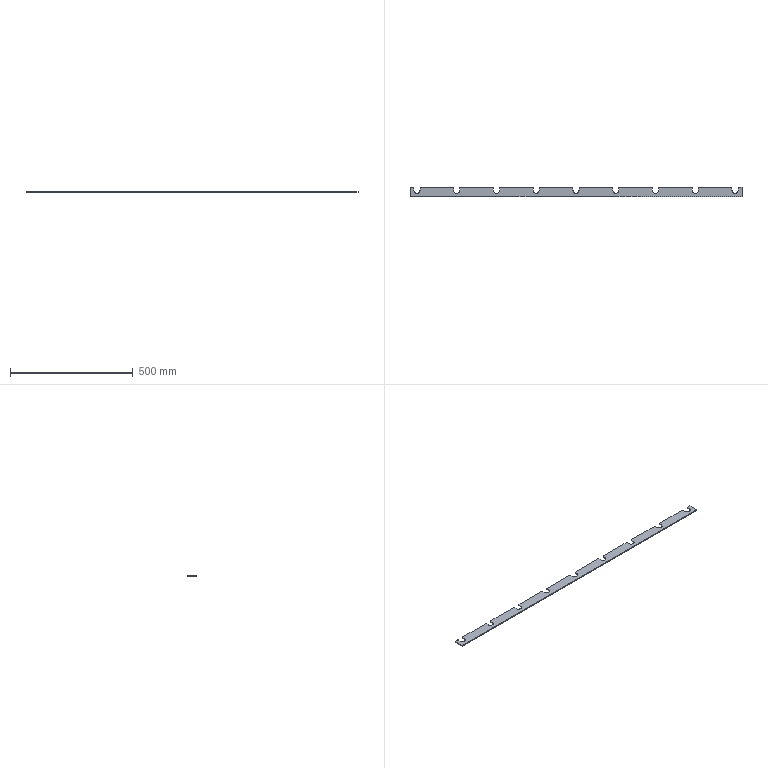Part | SolidWorks | features Extrusion 1, Fillet 1, ICE 1 | 1 solid | 60 faces | box 1350 x 40 x 4 mm | volume 195775 mm3 | plane 33 | cylinder 27 | commonest cylinder face diameters 6 x18 25 x9